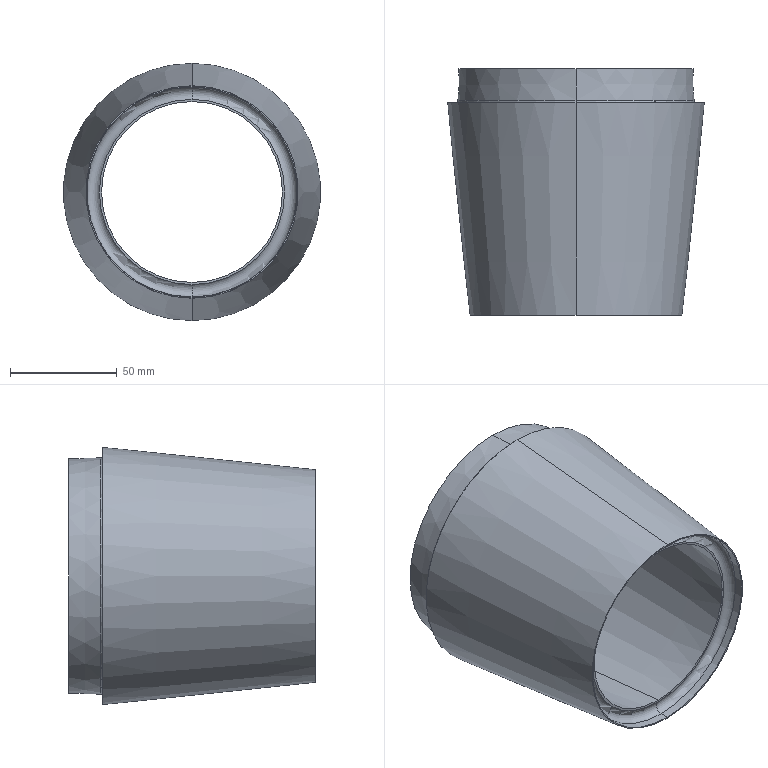Part | STEP file | rubber1 | 1 solid | 16 faces | box 120.71 x 115.719 x 120.71 mm | volume 254133 mm3 | cone 8 | torus 4 | plane 4
STEP:
#1=CARTESIAN_POINT('',(0.,-48.562,55.));
#2=VERTEX_POINT('',#1);
#3=CARTESIAN_POINT('',(0.,-48.562,-55.));
#4=VERTEX_POINT('',#3);
#5=CARTESIAN_POINT('',(0.,-48.562,0.));
#6=DIRECTION('',(0.,1.,0.));
#7=DIRECTION('',(0.,0.,1.));
#8=AXIS2_PLACEMENT_3D('',#5,#6,#7);
#9=CIRCLE('',#8,55.);
#10=EDGE_CURVE('',#2,#4,#9,.T.);
#11=ORIENTED_EDGE('',*,*,#10,.F.);
#12=CARTESIAN_POINT('',(0.,-63.492,55.447));
#13=VERTEX_POINT('',#12);
#14=CARTESIAN_POINT('',(0.,-63.492,55.447));
#15=DIRECTION('',(0.,-0.9996,0.02995));
#16=VECTOR('',#15,1000.);
#17=LINE('',#14,#16);
#18=EDGE_CURVE('',#2,#13,#17,.T.);
#19=ORIENTED_EDGE('',*,*,#18,.T.);
#20=CARTESIAN_POINT('',(0.,-63.492,-55.447));
#21=VERTEX_POINT('',#20);
#22=CARTESIAN_POINT('',(0.,-63.492,0.));
#23=DIRECTION('',(0.,1.,0.));
#24=DIRECTION('',(0.,0.,1.));
#25=AXIS2_PLACEMENT_3D('',#22,#23,#24);
#26=CIRCLE('',#25,55.447);
#27=EDGE_CURVE('',#13,#21,#26,.T.);
#28=ORIENTED_EDGE('',*,*,#27,.T.);
#29=CARTESIAN_POINT('',(0.,-63.492,-55.447));
#30=DIRECTION('',(0.,-0.9996,-0.02995));
#31=VECTOR('',#30,1000.);
#32=LINE('',#29,#31);
#33=EDGE_CURVE('',#4,#21,#32,.T.);
#34=ORIENTED_EDGE('',*,*,#33,.F.);
#35=EDGE_LOOP('',(#11,#19,#28,#34));
#36=FACE_OUTER_BOUND('',#35,.T.);
#37=CARTESIAN_POINT('',(0.,-63.492,0.));
#38=DIRECTION('',(0.,-1.,0.));
#39=DIRECTION('',(0.,0.,-1.));
#40=AXIS2_PLACEMENT_3D('',#37,#38,#39);
#41=CONICAL_SURFACE('',#40,55.447,0.02995);
#42=ADVANCED_FACE('',(#36),#41,.T.);
#43=CARTESIAN_POINT('',(0.,-63.492,0.));
#44=DIRECTION('',(0.,1.,0.));
#45=DIRECTION('',(0.,0.,1.));
#46=AXIS2_PLACEMENT_3D('',#43,#44,#45);
#47=CIRCLE('',#46,55.447);
#48=EDGE_CURVE('',#21,#13,#47,.T.);
#49=ORIENTED_EDGE('',*,*,#48,.F.);
#50=CARTESIAN_POINT('',(0.,-64.633,-59.855));
#51=VERTEX_POINT('',#50);
#52=CARTESIAN_POINT('',(0.,-63.421,-57.817));
#53=DIRECTION('',(1.,0.,0.));
#54=DIRECTION('',(0.,0.,-1.));
#55=AXIS2_PLACEMENT_3D('',#52,#53,#54);
#56=CIRCLE('',#55,2.371);
#57=EDGE_CURVE('',#21,#51,#56,.T.);
#58=ORIENTED_EDGE('',*,*,#57,.T.);
#59=CARTESIAN_POINT('',(0.,-64.633,59.855));
#60=VERTEX_POINT('',#59);
#61=CARTESIAN_POINT('',(0.,-64.633,0.));
#62=DIRECTION('',(0.,1.,0.));
#63=DIRECTION('',(0.,0.,1.));
#64=AXIS2_PLACEMENT_3D('',#61,#62,#63);
#65=CIRCLE('',#64,59.855);
#66=EDGE_CURVE('',#51,#60,#65,.T.);
#67=ORIENTED_EDGE('',*,*,#66,.T.);
#68=CARTESIAN_POINT('',(0.,-63.421,57.817));
#69=DIRECTION('',(-1.,0.,0.));
#70=DIRECTION('',(0.,0.,1.));
#71=AXIS2_PLACEMENT_3D('',#68,#69,#70);
#72=CIRCLE('',#71,2.371);
#73=EDGE_CURVE('',#13,#60,#72,.T.);
#74=ORIENTED_EDGE('',*,*,#73,.F.);
#75=EDGE_LOOP('',(#49,#58,#67,#74));
#76=FACE_OUTER_BOUND('',#75,.T.);
#77=CARTESIAN_POINT('',(0.,-63.421,0.));
#78=DIRECTION('',(0.,1.,0.));
#79=DIRECTION('',(0.,0.,1.));
#80=AXIS2_PLACEMENT_3D('',#77,#78,#79);
#81=TOROIDAL_SURFACE('',#80,57.817,2.371);
#82=ADVANCED_FACE('',(#76),#81,.F.);
#83=CARTESIAN_POINT('',(0.,-164.281,49.881));
#84=VERTEX_POINT('',#83);
#85=CARTESIAN_POINT('',(0.,-164.281,-49.881));
#86=VERTEX_POINT('',#85);
#87=CARTESIAN_POINT('',(0.,-164.281,0.));
#88=DIRECTION('',(0.,1.,0.));
#89=DIRECTION('',(0.,0.,1.));
#90=AXIS2_PLACEMENT_3D('',#87,#88,#89);
#91=CIRCLE('',#90,49.881);
#92=EDGE_CURVE('',#84,#86,#91,.T.);
#93=ORIENTED_EDGE('',*,*,#92,.T.);
#94=CARTESIAN_POINT('',(0.,-64.633,-60.355));
#95=VERTEX_POINT('',#94);
#96=CARTESIAN_POINT('',(0.,-164.281,-49.881));
#97=DIRECTION('',(0.,0.9945,-0.1045));
#98=VECTOR('',#97,1000.);
#99=LINE('',#96,#98);
#100=EDGE_CURVE('',#86,#95,#99,.T.);
#101=ORIENTED_EDGE('',*,*,#100,.T.);
#102=CARTESIAN_POINT('',(0.,-64.633,60.355));
#103=VERTEX_POINT('',#102);
#104=CARTESIAN_POINT('',(0.,-64.633,0.));
#105=DIRECTION('',(0.,1.,0.));
#106=DIRECTION('',(0.,0.,1.));
#107=AXIS2_PLACEMENT_3D('',#104,#105,#106);
#108=CIRCLE('',#107,60.355);
#109=EDGE_CURVE('',#103,#95,#108,.T.);
#110=ORIENTED_EDGE('',*,*,#109,.F.);
#111=CARTESIAN_POINT('',(0.,-164.281,49.881));
#112=DIRECTION('',(0.,0.9945,0.1045));
#113=VECTOR('',#112,1000.);
#114=LINE('',#111,#113);
#115=EDGE_CURVE('',#84,#103,#114,.T.);
#116=ORIENTED_EDGE('',*,*,#115,.F.);
#117=EDGE_LOOP('',(#93,#101,#110,#116));
#118=FACE_OUTER_BOUND('',#117,.T.);
#119=CARTESIAN_POINT('',(0.,-164.281,0.));
#120=DIRECTION('',(0.,1.,0.));
#121=DIRECTION('',(0.,0.,1.));
#122=AXIS2_PLACEMENT_3D('',#119,#120,#121);
#123=CONICAL_SURFACE('',#122,49.881,0.1047);
#124=ADVANCED_FACE('',(#118),#123,.T.);
#125=CARTESIAN_POINT('',(0.,-160.281,-49.296));
#126=VERTEX_POINT('',#125);
#127=CARTESIAN_POINT('',(0.,-160.281,49.296));
#128=VERTEX_POINT('',#127);
#129=CARTESIAN_POINT('',(0.,-160.281,0.));
#130=DIRECTION('',(0.,1.,0.));
#131=DIRECTION('',(0.,0.,1.));
#132=AXIS2_PLACEMENT_3D('',#129,#130,#131);
#133=CIRCLE('',#132,49.296);
#134=EDGE_CURVE('',#126,#128,#133,.T.);
#135=ORIENTED_EDGE('',*,*,#134,.T.);
#136=CARTESIAN_POINT('',(0.,-164.281,49.381));
#137=VERTEX_POINT('',#136);
#138=CARTESIAN_POINT('',(0.,-160.281,49.296));
#139=DIRECTION('',(0.,-0.9998,0.02127));
#140=VECTOR('',#139,1000.);
#141=LINE('',#138,#140);
#142=EDGE_CURVE('',#128,#137,#141,.T.);
#143=ORIENTED_EDGE('',*,*,#142,.T.);
#144=CARTESIAN_POINT('',(0.,-164.281,-49.381));
#145=VERTEX_POINT('',#144);
#146=CARTESIAN_POINT('',(0.,-164.281,0.));
#147=DIRECTION('',(0.,1.,0.));
#148=DIRECTION('',(0.,0.,1.));
#149=AXIS2_PLACEMENT_3D('',#146,#147,#148);
#150=CIRCLE('',#149,49.381);
#151=EDGE_CURVE('',#145,#137,#150,.T.);
#152=ORIENTED_EDGE('',*,*,#151,.F.);
#153=CARTESIAN_POINT('',(0.,-160.281,-49.296));
#154=DIRECTION('',(0.,-0.9998,-0.02127));
#155=VECTOR('',#154,1000.);
#156=LINE('',#153,#155);
#157=EDGE_CURVE('',#126,#145,#156,.T.);
#158=ORIENTED_EDGE('',*,*,#157,.F.);
#159=EDGE_LOOP('',(#135,#143,#152,#158));
#160=FACE_OUTER_BOUND('',#159,.T.);
#161=CARTESIAN_POINT('',(0.,-160.281,0.));
#162=DIRECTION('',(0.,-1.,0.));
#163=DIRECTION('',(0.,0.,-1.));
#164=AXIS2_PLACEMENT_3D('',#161,#162,#163);
#165=CONICAL_SURFACE('',#164,49.296,0.02127);
#166=ADVANCED_FACE('',(#160),#165,.F.);
#167=ORIENTED_EDGE('',*,*,#134,.F.);
#168=CARTESIAN_POINT('',(0.,-158.312,-43.465));
#169=VERTEX_POINT('',#168);
#170=CARTESIAN_POINT('',(0.,-160.351,-46.025));
#171=DIRECTION('',(1.,0.,0.));
#172=DIRECTION('',(0.,0.,-1.));
#173=AXIS2_PLACEMENT_3D('',#170,#171,#172);
#174=CIRCLE('',#173,3.272);
#175=EDGE_CURVE('',#126,#169,#174,.T.);
#176=ORIENTED_EDGE('',*,*,#175,.T.);
#177=CARTESIAN_POINT('',(0.,-158.312,43.465));
#178=VERTEX_POINT('',#177);
#179=CARTESIAN_POINT('',(0.,-158.312,0.));
#180=DIRECTION('',(0.,1.,0.));
#181=DIRECTION('',(0.,0.,1.));
#182=AXIS2_PLACEMENT_3D('',#179,#180,#181);
#183=CIRCLE('',#182,43.465);
#184=EDGE_CURVE('',#169,#178,#183,.T.);
#185=ORIENTED_EDGE('',*,*,#184,.T.);
#186=CARTESIAN_POINT('',(0.,-160.351,46.025));
#187=DIRECTION('',(-1.,0.,0.));
#188=DIRECTION('',(0.,0.,1.));
#189=AXIS2_PLACEMENT_3D('',#186,#187,#188);
#190=CIRCLE('',#189,3.272);
#191=EDGE_CURVE('',#128,#178,#190,.T.);
#192=ORIENTED_EDGE('',*,*,#191,.F.);
#193=EDGE_LOOP('',(#167,#176,#185,#192));
#194=FACE_OUTER_BOUND('',#193,.T.);
#195=CARTESIAN_POINT('',(0.,-160.351,0.));
#196=DIRECTION('',(0.,1.,0.));
#197=DIRECTION('',(0.,0.,1.));
#198=AXIS2_PLACEMENT_3D('',#195,#196,#197);
#199=TOROIDAL_SURFACE('',#198,46.025,3.272);
#200=ADVANCED_FACE('',(#194),#199,.F.);
#201=CARTESIAN_POINT('',(0.,-158.312,-42.465));
#202=VERTEX_POINT('',#201);
#203=CARTESIAN_POINT('',(0.,-158.312,42.465));
#204=VERTEX_POINT('',#203);
#205=CARTESIAN_POINT('',(0.,-158.312,0.));
#206=DIRECTION('',(0.,1.,0.));
#207=DIRECTION('',(0.,0.,1.));
#208=AXIS2_PLACEMENT_3D('',#205,#206,#207);
#209=CIRCLE('',#208,42.465);
#210=EDGE_CURVE('',#202,#204,#209,.T.);
#211=ORIENTED_EDGE('',*,*,#210,.F.);
#212=CARTESIAN_POINT('',(0.,-48.562,-54.));
#213=VERTEX_POINT('',#212);
#214=CARTESIAN_POINT('',(0.,-48.562,-54.));
#215=DIRECTION('',(0.,0.9945,-0.1045));
#216=VECTOR('',#215,1000.);
#217=LINE('',#214,#216);
#218=EDGE_CURVE('',#202,#213,#217,.T.);
#219=ORIENTED_EDGE('',*,*,#218,.T.);
#220=CARTESIAN_POINT('',(0.,-48.562,54.));
#221=VERTEX_POINT('',#220);
#222=CARTESIAN_POINT('',(0.,-48.562,0.));
#223=DIRECTION('',(0.,1.,0.));
#224=DIRECTION('',(0.,0.,1.));
#225=AXIS2_PLACEMENT_3D('',#222,#223,#224);
#226=CIRCLE('',#225,54.);
#227=EDGE_CURVE('',#213,#221,#226,.T.);
#228=ORIENTED_EDGE('',*,*,#227,.T.);
#229=CARTESIAN_POINT('',(0.,-48.562,54.));
#230=DIRECTION('',(0.,0.9945,0.1045));
#231=VECTOR('',#230,1000.);
#232=LINE('',#229,#231);
#233=EDGE_CURVE('',#204,#221,#232,.T.);
#234=ORIENTED_EDGE('',*,*,#233,.F.);
#235=EDGE_LOOP('',(#211,#219,#228,#234));
#236=FACE_OUTER_BOUND('',#235,.T.);
#237=CARTESIAN_POINT('',(0.,-48.562,0.));
#238=DIRECTION('',(0.,1.,0.));
#239=DIRECTION('',(0.,0.,1.));
#240=AXIS2_PLACEMENT_3D('',#237,#238,#239);
#241=CONICAL_SURFACE('',#240,54.,0.1047);
#242=ADVANCED_FACE('',(#236),#241,.F.);
#243=CARTESIAN_POINT('',(0.,-48.562,0.));
#244=DIRECTION('',(0.,1.,0.));
#245=DIRECTION('',(0.,0.,1.));
#246=AXIS2_PLACEMENT_3D('',#243,#244,#245);
#247=CIRCLE('',#246,54.);
#248=EDGE_CURVE('',#221,#213,#247,.T.);
#249=ORIENTED_EDGE('',*,*,#248,.F.);
#250=ORIENTED_EDGE('',*,*,#227,.F.);
#251=EDGE_LOOP('',(#249,#250));
#252=FACE_BOUND('',#251,.T.);
#253=CARTESIAN_POINT('',(0.,-48.562,0.));
#254=DIRECTION('',(0.,1.,0.));
#255=DIRECTION('',(0.,0.,1.));
#256=AXIS2_PLACEMENT_3D('',#253,#254,#255);
#257=CIRCLE('',#256,55.);
#258=EDGE_CURVE('',#4,#2,#257,.T.);
#259=ORIENTED_EDGE('',*,*,#258,.T.);
#260=ORIENTED_EDGE('',*,*,#10,.T.);
#261=EDGE_LOOP('',(#259,#260));
#262=FACE_OUTER_BOUND('',#261,.T.);
#263=CARTESIAN_POINT('',(54.,-48.562,0.));
#264=DIRECTION('',(0.,-1.,0.));
#265=DIRECTION('',(0.,0.,-1.));
#266=AXIS2_PLACEMENT_3D('',#263,#264,#265);
#267=PLANE('',#266);
#268=ADVANCED_FACE('',(#252,#262),#267,.F.);
#269=ORIENTED_EDGE('',*,*,#218,.F.);
#270=CARTESIAN_POINT('',(0.,-158.312,0.));
#271=DIRECTION('',(0.,1.,0.));
#272=DIRECTION('',(0.,0.,1.));
#273=AXIS2_PLACEMENT_3D('',#270,#271,#272);
#274=CIRCLE('',#273,42.465);
#275=EDGE_CURVE('',#204,#202,#274,.T.);
#276=ORIENTED_EDGE('',*,*,#275,.F.);
#277=ORIENTED_EDGE('',*,*,#233,.T.);
#278=ORIENTED_EDGE('',*,*,#248,.T.);
#279=EDGE_LOOP('',(#269,#276,#277,#278));
#280=FACE_OUTER_BOUND('',#279,.T.);
#281=CARTESIAN_POINT('',(0.,-48.562,0.));
#282=DIRECTION('',(0.,1.,0.));
#283=DIRECTION('',(0.,0.,1.));
#284=AXIS2_PLACEMENT_3D('',#281,#282,#283);
#285=CONICAL_SURFACE('',#284,54.,0.1047);
#286=ADVANCED_FACE('',(#280),#285,.F.);
#287=CARTESIAN_POINT('',(0.,-158.312,0.));
#288=DIRECTION('',(0.,1.,0.));
#289=DIRECTION('',(0.,0.,1.));
#290=AXIS2_PLACEMENT_3D('',#287,#288,#289);
#291=CIRCLE('',#290,43.465);
#292=EDGE_CURVE('',#178,#169,#291,.T.);
#293=ORIENTED_EDGE('',*,*,#292,.F.);
#294=ORIENTED_EDGE('',*,*,#184,.F.);
#295=EDGE_LOOP('',(#293,#294));
#296=FACE_OUTER_BOUND('',#295,.T.);
#297=ORIENTED_EDGE('',*,*,#275,.T.);
#298=ORIENTED_EDGE('',*,*,#210,.T.);
#299=EDGE_LOOP('',(#297,#298));
#300=FACE_BOUND('',#299,.T.);
#301=CARTESIAN_POINT('',(42.465,-158.312,0.));
#302=DIRECTION('',(0.,1.,0.));
#303=DIRECTION('',(0.,0.,1.));
#304=AXIS2_PLACEMENT_3D('',#301,#302,#303);
#305=PLANE('',#304);
#306=ADVANCED_FACE('',(#296,#300),#305,.F.);
#307=ORIENTED_EDGE('',*,*,#175,.F.);
#308=CARTESIAN_POINT('',(0.,-160.281,0.));
#309=DIRECTION('',(0.,1.,0.));
#310=DIRECTION('',(0.,0.,1.));
#311=AXIS2_PLACEMENT_3D('',#308,#309,#310);
#312=CIRCLE('',#311,49.296);
#313=EDGE_CURVE('',#128,#126,#312,.T.);
#314=ORIENTED_EDGE('',*,*,#313,.F.);
#315=ORIENTED_EDGE('',*,*,#191,.T.);
#316=ORIENTED_EDGE('',*,*,#292,.T.);
#317=EDGE_LOOP('',(#307,#314,#315,#316));
#318=FACE_OUTER_BOUND('',#317,.T.);
#319=CARTESIAN_POINT('',(0.,-160.351,0.));
#320=DIRECTION('',(0.,1.,0.));
#321=DIRECTION('',(0.,0.,1.));
#322=AXIS2_PLACEMENT_3D('',#319,#320,#321);
#323=TOROIDAL_SURFACE('',#322,46.025,3.272);
#324=ADVANCED_FACE('',(#318),#323,.F.);
#325=ORIENTED_EDGE('',*,*,#142,.F.);
#326=ORIENTED_EDGE('',*,*,#313,.T.);
#327=ORIENTED_EDGE('',*,*,#157,.T.);
#328=CARTESIAN_POINT('',(0.,-164.281,0.));
#329=DIRECTION('',(0.,1.,0.));
#330=DIRECTION('',(0.,0.,1.));
#331=AXIS2_PLACEMENT_3D('',#328,#329,#330);
#332=CIRCLE('',#331,49.381);
#333=EDGE_CURVE('',#137,#145,#332,.T.);
#334=ORIENTED_EDGE('',*,*,#333,.F.);
#335=EDGE_LOOP('',(#325,#326,#327,#334));
#336=FACE_OUTER_BOUND('',#335,.T.);
#337=CARTESIAN_POINT('',(0.,-160.281,0.));
#338=DIRECTION('',(0.,-1.,0.));
#339=DIRECTION('',(0.,0.,-1.));
#340=AXIS2_PLACEMENT_3D('',#337,#338,#339);
#341=CONICAL_SURFACE('',#340,49.296,0.02127);
#342=ADVANCED_FACE('',(#336),#341,.F.);
#343=ORIENTED_EDGE('',*,*,#92,.F.);
#344=CARTESIAN_POINT('',(0.,-164.281,0.));
#345=DIRECTION('',(0.,1.,0.));
#346=DIRECTION('',(0.,0.,1.));
#347=AXIS2_PLACEMENT_3D('',#344,#345,#346);
#348=CIRCLE('',#347,49.881);
#349=EDGE_CURVE('',#86,#84,#348,.T.);
#350=ORIENTED_EDGE('',*,*,#349,.F.);
#351=EDGE_LOOP('',(#343,#350));
#352=FACE_OUTER_BOUND('',#351,.T.);
#353=ORIENTED_EDGE('',*,*,#151,.T.);
#354=ORIENTED_EDGE('',*,*,#333,.T.);
#355=EDGE_LOOP('',(#353,#354));
#356=FACE_BOUND('',#355,.T.);
#357=CARTESIAN_POINT('',(49.881,-164.281,0.));
#358=DIRECTION('',(0.,1.,0.));
#359=DIRECTION('',(0.,0.,1.));
#360=AXIS2_PLACEMENT_3D('',#357,#358,#359);
#361=PLANE('',#360);
#362=ADVANCED_FACE('',(#352,#356),#361,.F.);
#363=ORIENTED_EDGE('',*,*,#100,.F.);
#364=ORIENTED_EDGE('',*,*,#349,.T.);
#365=ORIENTED_EDGE('',*,*,#115,.T.);
#366=CARTESIAN_POINT('',(0.,-64.633,0.));
#367=DIRECTION('',(0.,1.,0.));
#368=DIRECTION('',(0.,0.,1.));
#369=AXIS2_PLACEMENT_3D('',#366,#367,#368);
#370=CIRCLE('',#369,60.355);
#371=EDGE_CURVE('',#95,#103,#370,.T.);
#372=ORIENTED_EDGE('',*,*,#371,.F.);
#373=EDGE_LOOP('',(#363,#364,#365,#372));
#374=FACE_OUTER_BOUND('',#373,.T.);
#375=CARTESIAN_POINT('',(0.,-164.281,0.));
#376=DIRECTION('',(0.,1.,0.));
#377=DIRECTION('',(0.,0.,1.));
#378=AXIS2_PLACEMENT_3D('',#375,#376,#377);
#379=CONICAL_SURFACE('',#378,49.881,0.1047);
#380=ADVANCED_FACE('',(#374),#379,.T.);
#381=CARTESIAN_POINT('',(0.,-64.633,0.));
#382=DIRECTION('',(0.,1.,0.));
#383=DIRECTION('',(0.,0.,1.));
#384=AXIS2_PLACEMENT_3D('',#381,#382,#383);
#385=CIRCLE('',#384,59.855);
#386=EDGE_CURVE('',#60,#51,#385,.T.);
#387=ORIENTED_EDGE('',*,*,#386,.F.);
#388=ORIENTED_EDGE('',*,*,#66,.F.);
#389=EDGE_LOOP('',(#387,#388));
#390=FACE_BOUND('',#389,.T.);
#391=ORIENTED_EDGE('',*,*,#109,.T.);
#392=ORIENTED_EDGE('',*,*,#371,.T.);
#393=EDGE_LOOP('',(#391,#392));
#394=FACE_OUTER_BOUND('',#393,.T.);
#395=CARTESIAN_POINT('',(60.355,-64.633,0.));
#396=DIRECTION('',(0.,-1.,0.));
#397=DIRECTION('',(0.,0.,-1.));
#398=AXIS2_PLACEMENT_3D('',#395,#396,#397);
#399=PLANE('',#398);
#400=ADVANCED_FACE('',(#390,#394),#399,.F.);
#401=ORIENTED_EDGE('',*,*,#57,.F.);
#402=ORIENTED_EDGE('',*,*,#27,.F.);
#403=ORIENTED_EDGE('',*,*,#73,.T.);
#404=ORIENTED_EDGE('',*,*,#386,.T.);
#405=EDGE_LOOP('',(#401,#402,#403,#404));
#406=FACE_OUTER_BOUND('',#405,.T.);
#407=CARTESIAN_POINT('',(0.,-63.421,0.));
#408=DIRECTION('',(0.,1.,0.));
#409=DIRECTION('',(0.,0.,1.));
#410=AXIS2_PLACEMENT_3D('',#407,#408,#409);
#411=TOROIDAL_SURFACE('',#410,57.817,2.371);
#412=ADVANCED_FACE('',(#406),#411,.F.);
#413=ORIENTED_EDGE('',*,*,#18,.F.);
#414=ORIENTED_EDGE('',*,*,#258,.F.);
#415=ORIENTED_EDGE('',*,*,#33,.T.);
#416=ORIENTED_EDGE('',*,*,#48,.T.);
#417=EDGE_LOOP('',(#413,#414,#415,#416));
#418=FACE_OUTER_BOUND('',#417,.T.);
#419=CARTESIAN_POINT('',(0.,-63.492,0.));
#420=DIRECTION('',(0.,-1.,0.));
#421=DIRECTION('',(0.,0.,-1.));
#422=AXIS2_PLACEMENT_3D('',#419,#420,#421);
#423=CONICAL_SURFACE('',#422,55.447,0.02995);
#424=ADVANCED_FACE('',(#418),#423,.T.);
#425=CLOSED_SHELL('',(#42,#82,#124,#166,#200,#242,#268,#286,#306,#324,#342,#362,#380,#400,#412,#424));
#426=MANIFOLD_SOLID_BREP('',#425);
#427=CARTESIAN_POINT('',(0.,0.,0.));
#428=DIRECTION('',(0.,0.,1.));
#429=DIRECTION('',(1.,0.,0.));
#430=AXIS2_PLACEMENT_3D('',#427,#428,#429);
#431=(LENGTH_UNIT()NAMED_UNIT(*)SI_UNIT(.MILLI.,.METRE.));
#432=UNCERTAINTY_MEASURE_WITH_UNIT(LENGTH_MEASURE(0.00001),#431,'','');
#433=(NAMED_UNIT(*)PLANE_ANGLE_UNIT()SI_UNIT($,.RADIAN.));
#434=(NAMED_UNIT(*)SI_UNIT($,.STERADIAN.)SOLID_ANGLE_UNIT());
#435=(GEOMETRIC_REPRESENTATION_CONTEXT(3)GLOBAL_UNCERTAINTY_ASSIGNED_CONTEXT((#432))GLOBAL_UNIT_ASSIGNED_CONTEXT((#431,#433,#434))REPRESENTATION_CONTEXT('',''));
#436=ADVANCED_BREP_SHAPE_REPRESENTATION('',(#426,#430),#435);